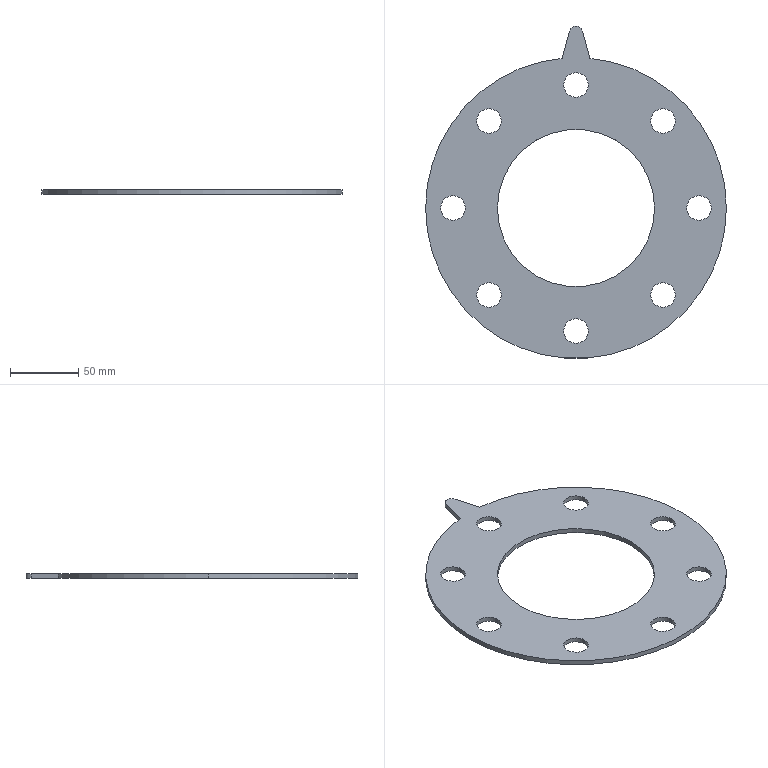Part | SolidWorks | features Extrusion 1 | 1 solid | 26 faces | box 220 x 243.233 x 3.5 mm | volume 90689 mm3 | cylinder 22 | plane 4 | commonest cylinder face diameters 18 x16 220 x3 115 x2 10 x1
STEP:
#1=CARTESIAN_POINT('',(-72.64,63.64,3.5));
#2=VERTEX_POINT('',#1);
#3=CARTESIAN_POINT('',(-54.64,63.64,3.5));
#4=VERTEX_POINT('',#3);
#5=CARTESIAN_POINT('',(-63.64,63.64,3.5));
#6=DIRECTION('',(0.,0.,1.));
#7=DIRECTION('',(1.,0.,0.));
#8=AXIS2_PLACEMENT_3D('',#5,#6,#7);
#9=CIRCLE('',#8,9.);
#10=EDGE_CURVE('',#2,#4,#9,.T.);
#11=ORIENTED_EDGE('',*,*,#10,.T.);
#12=CARTESIAN_POINT('',(-54.64,63.64,0.));
#13=VERTEX_POINT('',#12);
#14=CARTESIAN_POINT('',(-54.64,63.64,3.5));
#15=DIRECTION('',(0.,0.,-1.));
#16=VECTOR('',#15,1000.);
#17=LINE('',#14,#16);
#18=EDGE_CURVE('',#4,#13,#17,.T.);
#19=ORIENTED_EDGE('',*,*,#18,.T.);
#20=CARTESIAN_POINT('',(-72.64,63.64,0.));
#21=VERTEX_POINT('',#20);
#22=CARTESIAN_POINT('',(-63.64,63.64,0.));
#23=DIRECTION('',(0.,0.,1.));
#24=DIRECTION('',(1.,0.,0.));
#25=AXIS2_PLACEMENT_3D('',#22,#23,#24);
#26=CIRCLE('',#25,9.);
#27=EDGE_CURVE('',#21,#13,#26,.T.);
#28=ORIENTED_EDGE('',*,*,#27,.F.);
#29=CARTESIAN_POINT('',(-72.64,63.64,3.5));
#30=DIRECTION('',(0.,0.,-1.));
#31=VECTOR('',#30,1000.);
#32=LINE('',#29,#31);
#33=EDGE_CURVE('',#2,#21,#32,.T.);
#34=ORIENTED_EDGE('',*,*,#33,.F.);
#35=EDGE_LOOP('',(#11,#19,#28,#34));
#36=FACE_OUTER_BOUND('',#35,.T.);
#37=CARTESIAN_POINT('',(-63.64,63.64,3.5));
#38=DIRECTION('',(0.,0.,-1.));
#39=DIRECTION('',(-1.,0.,0.));
#40=AXIS2_PLACEMENT_3D('',#37,#38,#39);
#41=CYLINDRICAL_SURFACE('',#40,9.);
#42=ADVANCED_FACE('',(#36),#41,.F.);
#43=CARTESIAN_POINT('',(-99.,0.,3.5));
#44=VERTEX_POINT('',#43);
#45=CARTESIAN_POINT('',(-81.,0.,3.5));
#46=VERTEX_POINT('',#45);
#47=CARTESIAN_POINT('',(-90.,0.,3.5));
#48=DIRECTION('',(0.,0.,1.));
#49=DIRECTION('',(1.,0.,0.));
#50=AXIS2_PLACEMENT_3D('',#47,#48,#49);
#51=CIRCLE('',#50,9.);
#52=EDGE_CURVE('',#44,#46,#51,.T.);
#53=ORIENTED_EDGE('',*,*,#52,.T.);
#54=CARTESIAN_POINT('',(-81.,0.,0.));
#55=VERTEX_POINT('',#54);
#56=CARTESIAN_POINT('',(-81.,0.,3.5));
#57=DIRECTION('',(0.,0.,-1.));
#58=VECTOR('',#57,1000.);
#59=LINE('',#56,#58);
#60=EDGE_CURVE('',#46,#55,#59,.T.);
#61=ORIENTED_EDGE('',*,*,#60,.T.);
#62=CARTESIAN_POINT('',(-99.,0.,0.));
#63=VERTEX_POINT('',#62);
#64=CARTESIAN_POINT('',(-90.,0.,0.));
#65=DIRECTION('',(0.,0.,1.));
#66=DIRECTION('',(1.,0.,0.));
#67=AXIS2_PLACEMENT_3D('',#64,#65,#66);
#68=CIRCLE('',#67,9.);
#69=EDGE_CURVE('',#63,#55,#68,.T.);
#70=ORIENTED_EDGE('',*,*,#69,.F.);
#71=CARTESIAN_POINT('',(-99.,0.,3.5));
#72=DIRECTION('',(0.,0.,-1.));
#73=VECTOR('',#72,1000.);
#74=LINE('',#71,#73);
#75=EDGE_CURVE('',#44,#63,#74,.T.);
#76=ORIENTED_EDGE('',*,*,#75,.F.);
#77=EDGE_LOOP('',(#53,#61,#70,#76));
#78=FACE_OUTER_BOUND('',#77,.T.);
#79=CARTESIAN_POINT('',(-90.,0.,3.5));
#80=DIRECTION('',(0.,0.,-1.));
#81=DIRECTION('',(-1.,0.,0.));
#82=AXIS2_PLACEMENT_3D('',#79,#80,#81);
#83=CYLINDRICAL_SURFACE('',#82,9.);
#84=ADVANCED_FACE('',(#78),#83,.F.);
#85=CARTESIAN_POINT('',(-72.64,-63.64,3.5));
#86=VERTEX_POINT('',#85);
#87=CARTESIAN_POINT('',(-54.64,-63.64,3.5));
#88=VERTEX_POINT('',#87);
#89=CARTESIAN_POINT('',(-63.64,-63.64,3.5));
#90=DIRECTION('',(0.,0.,1.));
#91=DIRECTION('',(1.,0.,0.));
#92=AXIS2_PLACEMENT_3D('',#89,#90,#91);
#93=CIRCLE('',#92,9.);
#94=EDGE_CURVE('',#86,#88,#93,.T.);
#95=ORIENTED_EDGE('',*,*,#94,.T.);
#96=CARTESIAN_POINT('',(-54.64,-63.64,0.));
#97=VERTEX_POINT('',#96);
#98=CARTESIAN_POINT('',(-54.64,-63.64,3.5));
#99=DIRECTION('',(0.,0.,-1.));
#100=VECTOR('',#99,1000.);
#101=LINE('',#98,#100);
#102=EDGE_CURVE('',#88,#97,#101,.T.);
#103=ORIENTED_EDGE('',*,*,#102,.T.);
#104=CARTESIAN_POINT('',(-72.64,-63.64,0.));
#105=VERTEX_POINT('',#104);
#106=CARTESIAN_POINT('',(-63.64,-63.64,0.));
#107=DIRECTION('',(0.,0.,1.));
#108=DIRECTION('',(1.,0.,0.));
#109=AXIS2_PLACEMENT_3D('',#106,#107,#108);
#110=CIRCLE('',#109,9.);
#111=EDGE_CURVE('',#105,#97,#110,.T.);
#112=ORIENTED_EDGE('',*,*,#111,.F.);
#113=CARTESIAN_POINT('',(-72.64,-63.64,3.5));
#114=DIRECTION('',(0.,0.,-1.));
#115=VECTOR('',#114,1000.);
#116=LINE('',#113,#115);
#117=EDGE_CURVE('',#86,#105,#116,.T.);
#118=ORIENTED_EDGE('',*,*,#117,.F.);
#119=EDGE_LOOP('',(#95,#103,#112,#118));
#120=FACE_OUTER_BOUND('',#119,.T.);
#121=CARTESIAN_POINT('',(-63.64,-63.64,3.5));
#122=DIRECTION('',(0.,0.,-1.));
#123=DIRECTION('',(-1.,0.,0.));
#124=AXIS2_PLACEMENT_3D('',#121,#122,#123);
#125=CYLINDRICAL_SURFACE('',#124,9.);
#126=ADVANCED_FACE('',(#120),#125,.F.);
#127=CARTESIAN_POINT('',(-9.,-90.,3.5));
#128=VERTEX_POINT('',#127);
#129=CARTESIAN_POINT('',(9.,-90.,3.5));
#130=VERTEX_POINT('',#129);
#131=CARTESIAN_POINT('',(0.,-90.,3.5));
#132=DIRECTION('',(0.,0.,1.));
#133=DIRECTION('',(1.,0.,0.));
#134=AXIS2_PLACEMENT_3D('',#131,#132,#133);
#135=CIRCLE('',#134,9.);
#136=EDGE_CURVE('',#128,#130,#135,.T.);
#137=ORIENTED_EDGE('',*,*,#136,.T.);
#138=CARTESIAN_POINT('',(9.,-90.,0.));
#139=VERTEX_POINT('',#138);
#140=CARTESIAN_POINT('',(9.,-90.,3.5));
#141=DIRECTION('',(0.,0.,-1.));
#142=VECTOR('',#141,1000.);
#143=LINE('',#140,#142);
#144=EDGE_CURVE('',#130,#139,#143,.T.);
#145=ORIENTED_EDGE('',*,*,#144,.T.);
#146=CARTESIAN_POINT('',(-9.,-90.,0.));
#147=VERTEX_POINT('',#146);
#148=CARTESIAN_POINT('',(0.,-90.,0.));
#149=DIRECTION('',(0.,0.,1.));
#150=DIRECTION('',(1.,0.,0.));
#151=AXIS2_PLACEMENT_3D('',#148,#149,#150);
#152=CIRCLE('',#151,9.);
#153=EDGE_CURVE('',#147,#139,#152,.T.);
#154=ORIENTED_EDGE('',*,*,#153,.F.);
#155=CARTESIAN_POINT('',(-9.,-90.,3.5));
#156=DIRECTION('',(0.,0.,-1.));
#157=VECTOR('',#156,1000.);
#158=LINE('',#155,#157);
#159=EDGE_CURVE('',#128,#147,#158,.T.);
#160=ORIENTED_EDGE('',*,*,#159,.F.);
#161=EDGE_LOOP('',(#137,#145,#154,#160));
#162=FACE_OUTER_BOUND('',#161,.T.);
#163=CARTESIAN_POINT('',(0.,-90.,3.5));
#164=DIRECTION('',(0.,0.,-1.));
#165=DIRECTION('',(-1.,0.,0.));
#166=AXIS2_PLACEMENT_3D('',#163,#164,#165);
#167=CYLINDRICAL_SURFACE('',#166,9.);
#168=ADVANCED_FACE('',(#162),#167,.F.);
#169=CARTESIAN_POINT('',(54.64,-63.64,3.5));
#170=VERTEX_POINT('',#169);
#171=CARTESIAN_POINT('',(72.64,-63.64,3.5));
#172=VERTEX_POINT('',#171);
#173=CARTESIAN_POINT('',(63.64,-63.64,3.5));
#174=DIRECTION('',(0.,0.,1.));
#175=DIRECTION('',(1.,0.,0.));
#176=AXIS2_PLACEMENT_3D('',#173,#174,#175);
#177=CIRCLE('',#176,9.);
#178=EDGE_CURVE('',#170,#172,#177,.T.);
#179=ORIENTED_EDGE('',*,*,#178,.T.);
#180=CARTESIAN_POINT('',(72.64,-63.64,0.));
#181=VERTEX_POINT('',#180);
#182=CARTESIAN_POINT('',(72.64,-63.64,3.5));
#183=DIRECTION('',(0.,0.,-1.));
#184=VECTOR('',#183,1000.);
#185=LINE('',#182,#184);
#186=EDGE_CURVE('',#172,#181,#185,.T.);
#187=ORIENTED_EDGE('',*,*,#186,.T.);
#188=CARTESIAN_POINT('',(54.64,-63.64,0.));
#189=VERTEX_POINT('',#188);
#190=CARTESIAN_POINT('',(63.64,-63.64,0.));
#191=DIRECTION('',(0.,0.,1.));
#192=DIRECTION('',(1.,0.,0.));
#193=AXIS2_PLACEMENT_3D('',#190,#191,#192);
#194=CIRCLE('',#193,9.);
#195=EDGE_CURVE('',#189,#181,#194,.T.);
#196=ORIENTED_EDGE('',*,*,#195,.F.);
#197=CARTESIAN_POINT('',(54.64,-63.64,3.5));
#198=DIRECTION('',(0.,0.,-1.));
#199=VECTOR('',#198,1000.);
#200=LINE('',#197,#199);
#201=EDGE_CURVE('',#170,#189,#200,.T.);
#202=ORIENTED_EDGE('',*,*,#201,.F.);
#203=EDGE_LOOP('',(#179,#187,#196,#202));
#204=FACE_OUTER_BOUND('',#203,.T.);
#205=CARTESIAN_POINT('',(63.64,-63.64,3.5));
#206=DIRECTION('',(0.,0.,-1.));
#207=DIRECTION('',(-1.,0.,0.));
#208=AXIS2_PLACEMENT_3D('',#205,#206,#207);
#209=CYLINDRICAL_SURFACE('',#208,9.);
#210=ADVANCED_FACE('',(#204),#209,.F.);
#211=CARTESIAN_POINT('',(81.,0.,3.5));
#212=VERTEX_POINT('',#211);
#213=CARTESIAN_POINT('',(99.,0.,3.5));
#214=VERTEX_POINT('',#213);
#215=CARTESIAN_POINT('',(90.,0.,3.5));
#216=DIRECTION('',(0.,0.,1.));
#217=DIRECTION('',(1.,0.,0.));
#218=AXIS2_PLACEMENT_3D('',#215,#216,#217);
#219=CIRCLE('',#218,9.);
#220=EDGE_CURVE('',#212,#214,#219,.T.);
#221=ORIENTED_EDGE('',*,*,#220,.T.);
#222=CARTESIAN_POINT('',(99.,0.,0.));
#223=VERTEX_POINT('',#222);
#224=CARTESIAN_POINT('',(99.,0.,3.5));
#225=DIRECTION('',(0.,0.,-1.));
#226=VECTOR('',#225,1000.);
#227=LINE('',#224,#226);
#228=EDGE_CURVE('',#214,#223,#227,.T.);
#229=ORIENTED_EDGE('',*,*,#228,.T.);
#230=CARTESIAN_POINT('',(81.,0.,0.));
#231=VERTEX_POINT('',#230);
#232=CARTESIAN_POINT('',(90.,0.,0.));
#233=DIRECTION('',(0.,0.,1.));
#234=DIRECTION('',(1.,0.,0.));
#235=AXIS2_PLACEMENT_3D('',#232,#233,#234);
#236=CIRCLE('',#235,9.);
#237=EDGE_CURVE('',#231,#223,#236,.T.);
#238=ORIENTED_EDGE('',*,*,#237,.F.);
#239=CARTESIAN_POINT('',(81.,0.,3.5));
#240=DIRECTION('',(0.,0.,-1.));
#241=VECTOR('',#240,1000.);
#242=LINE('',#239,#241);
#243=EDGE_CURVE('',#212,#231,#242,.T.);
#244=ORIENTED_EDGE('',*,*,#243,.F.);
#245=EDGE_LOOP('',(#221,#229,#238,#244));
#246=FACE_OUTER_BOUND('',#245,.T.);
#247=CARTESIAN_POINT('',(90.,0.,3.5));
#248=DIRECTION('',(0.,0.,-1.));
#249=DIRECTION('',(-1.,0.,0.));
#250=AXIS2_PLACEMENT_3D('',#247,#248,#249);
#251=CYLINDRICAL_SURFACE('',#250,9.);
#252=ADVANCED_FACE('',(#246),#251,.F.);
#253=CARTESIAN_POINT('',(54.64,63.64,3.5));
#254=VERTEX_POINT('',#253);
#255=CARTESIAN_POINT('',(72.64,63.64,3.5));
#256=VERTEX_POINT('',#255);
#257=CARTESIAN_POINT('',(63.64,63.64,3.5));
#258=DIRECTION('',(0.,0.,1.));
#259=DIRECTION('',(1.,0.,0.));
#260=AXIS2_PLACEMENT_3D('',#257,#258,#259);
#261=CIRCLE('',#260,9.);
#262=EDGE_CURVE('',#254,#256,#261,.T.);
#263=ORIENTED_EDGE('',*,*,#262,.T.);
#264=CARTESIAN_POINT('',(72.64,63.64,0.));
#265=VERTEX_POINT('',#264);
#266=CARTESIAN_POINT('',(72.64,63.64,3.5));
#267=DIRECTION('',(0.,0.,-1.));
#268=VECTOR('',#267,1000.);
#269=LINE('',#266,#268);
#270=EDGE_CURVE('',#256,#265,#269,.T.);
#271=ORIENTED_EDGE('',*,*,#270,.T.);
#272=CARTESIAN_POINT('',(54.64,63.64,0.));
#273=VERTEX_POINT('',#272);
#274=CARTESIAN_POINT('',(63.64,63.64,0.));
#275=DIRECTION('',(0.,0.,1.));
#276=DIRECTION('',(1.,0.,0.));
#277=AXIS2_PLACEMENT_3D('',#274,#275,#276);
#278=CIRCLE('',#277,9.);
#279=EDGE_CURVE('',#273,#265,#278,.T.);
#280=ORIENTED_EDGE('',*,*,#279,.F.);
#281=CARTESIAN_POINT('',(54.64,63.64,3.5));
#282=DIRECTION('',(0.,0.,-1.));
#283=VECTOR('',#282,1000.);
#284=LINE('',#281,#283);
#285=EDGE_CURVE('',#254,#273,#284,.T.);
#286=ORIENTED_EDGE('',*,*,#285,.F.);
#287=EDGE_LOOP('',(#263,#271,#280,#286));
#288=FACE_OUTER_BOUND('',#287,.T.);
#289=CARTESIAN_POINT('',(63.64,63.64,3.5));
#290=DIRECTION('',(0.,0.,-1.));
#291=DIRECTION('',(-1.,0.,0.));
#292=AXIS2_PLACEMENT_3D('',#289,#290,#291);
#293=CYLINDRICAL_SURFACE('',#292,9.);
#294=ADVANCED_FACE('',(#288),#293,.F.);
#295=CARTESIAN_POINT('',(-9.,90.,3.5));
#296=VERTEX_POINT('',#295);
#297=CARTESIAN_POINT('',(9.,90.,3.5));
#298=VERTEX_POINT('',#297);
#299=CARTESIAN_POINT('',(0.,90.,3.5));
#300=DIRECTION('',(0.,0.,1.));
#301=DIRECTION('',(1.,0.,0.));
#302=AXIS2_PLACEMENT_3D('',#299,#300,#301);
#303=CIRCLE('',#302,9.);
#304=EDGE_CURVE('',#296,#298,#303,.T.);
#305=ORIENTED_EDGE('',*,*,#304,.T.);
#306=CARTESIAN_POINT('',(9.,90.,0.));
#307=VERTEX_POINT('',#306);
#308=CARTESIAN_POINT('',(9.,90.,3.5));
#309=DIRECTION('',(0.,0.,-1.));
#310=VECTOR('',#309,1000.);
#311=LINE('',#308,#310);
#312=EDGE_CURVE('',#298,#307,#311,.T.);
#313=ORIENTED_EDGE('',*,*,#312,.T.);
#314=CARTESIAN_POINT('',(-9.,90.,0.));
#315=VERTEX_POINT('',#314);
#316=CARTESIAN_POINT('',(0.,90.,0.));
#317=DIRECTION('',(0.,0.,1.));
#318=DIRECTION('',(1.,0.,0.));
#319=AXIS2_PLACEMENT_3D('',#316,#317,#318);
#320=CIRCLE('',#319,9.);
#321=EDGE_CURVE('',#315,#307,#320,.T.);
#322=ORIENTED_EDGE('',*,*,#321,.F.);
#323=CARTESIAN_POINT('',(-9.,90.,3.5));
#324=DIRECTION('',(0.,0.,-1.));
#325=VECTOR('',#324,1000.);
#326=LINE('',#323,#325);
#327=EDGE_CURVE('',#296,#315,#326,.T.);
#328=ORIENTED_EDGE('',*,*,#327,.F.);
#329=EDGE_LOOP('',(#305,#313,#322,#328));
#330=FACE_OUTER_BOUND('',#329,.T.);
#331=CARTESIAN_POINT('',(0.,90.,3.5));
#332=DIRECTION('',(0.,0.,-1.));
#333=DIRECTION('',(-1.,0.,0.));
#334=AXIS2_PLACEMENT_3D('',#331,#332,#333);
#335=CYLINDRICAL_SURFACE('',#334,9.);
#336=ADVANCED_FACE('',(#330),#335,.F.);
#337=CARTESIAN_POINT('',(-57.5,0.,3.5));
#338=VERTEX_POINT('',#337);
#339=CARTESIAN_POINT('',(57.5,0.,3.5));
#340=VERTEX_POINT('',#339);
#341=CARTESIAN_POINT('',(0.,0.,3.5));
#342=DIRECTION('',(0.,0.,1.));
#343=DIRECTION('',(1.,0.,0.));
#344=AXIS2_PLACEMENT_3D('',#341,#342,#343);
#345=CIRCLE('',#344,57.5);
#346=EDGE_CURVE('',#338,#340,#345,.T.);
#347=ORIENTED_EDGE('',*,*,#346,.T.);
#348=CARTESIAN_POINT('',(57.5,0.,0.));
#349=VERTEX_POINT('',#348);
#350=CARTESIAN_POINT('',(57.5,0.,3.5));
#351=DIRECTION('',(0.,0.,-1.));
#352=VECTOR('',#351,1000.);
#353=LINE('',#350,#352);
#354=EDGE_CURVE('',#340,#349,#353,.T.);
#355=ORIENTED_EDGE('',*,*,#354,.T.);
#356=CARTESIAN_POINT('',(-57.5,0.,0.));
#357=VERTEX_POINT('',#356);
#358=CARTESIAN_POINT('',(0.,0.,0.));
#359=DIRECTION('',(0.,0.,1.));
#360=DIRECTION('',(1.,0.,0.));
#361=AXIS2_PLACEMENT_3D('',#358,#359,#360);
#362=CIRCLE('',#361,57.5);
#363=EDGE_CURVE('',#357,#349,#362,.T.);
#364=ORIENTED_EDGE('',*,*,#363,.F.);
#365=CARTESIAN_POINT('',(-57.5,0.,3.5));
#366=DIRECTION('',(0.,0.,-1.));
#367=VECTOR('',#366,1000.);
#368=LINE('',#365,#367);
#369=EDGE_CURVE('',#338,#357,#368,.T.);
#370=ORIENTED_EDGE('',*,*,#369,.F.);
#371=EDGE_LOOP('',(#347,#355,#364,#370));
#372=FACE_OUTER_BOUND('',#371,.T.);
#373=CARTESIAN_POINT('',(0.,0.,3.5));
#374=DIRECTION('',(0.,0.,-1.));
#375=DIRECTION('',(-1.,0.,0.));
#376=AXIS2_PLACEMENT_3D('',#373,#374,#375);
#377=CYLINDRICAL_SURFACE('',#376,57.5);
#378=ADVANCED_FACE('',(#372),#377,.F.);
#379=CARTESIAN_POINT('',(110.,0.,3.5));
#380=VERTEX_POINT('',#379);
#381=CARTESIAN_POINT('',(10.189,109.527,3.5));
#382=VERTEX_POINT('',#381);
#383=CARTESIAN_POINT('',(0.,0.,3.5));
#384=DIRECTION('',(0.,0.,1.));
#385=DIRECTION('',(1.,0.,0.));
#386=AXIS2_PLACEMENT_3D('',#383,#384,#385);
#387=CIRCLE('',#386,110.);
#388=EDGE_CURVE('',#380,#382,#387,.T.);
#389=ORIENTED_EDGE('',*,*,#388,.F.);
#390=CARTESIAN_POINT('',(110.,0.,0.));
#391=VERTEX_POINT('',#390);
#392=CARTESIAN_POINT('',(110.,0.,3.5));
#393=DIRECTION('',(0.,0.,-1.));
#394=VECTOR('',#393,1000.);
#395=LINE('',#392,#394);
#396=EDGE_CURVE('',#380,#391,#395,.T.);
#397=ORIENTED_EDGE('',*,*,#396,.T.);
#398=CARTESIAN_POINT('',(10.189,109.527,0.));
#399=VERTEX_POINT('',#398);
#400=CARTESIAN_POINT('',(0.,0.,0.));
#401=DIRECTION('',(0.,0.,1.));
#402=DIRECTION('',(1.,0.,0.));
#403=AXIS2_PLACEMENT_3D('',#400,#401,#402);
#404=CIRCLE('',#403,110.);
#405=EDGE_CURVE('',#391,#399,#404,.T.);
#406=ORIENTED_EDGE('',*,*,#405,.T.);
#407=CARTESIAN_POINT('',(10.189,109.527,3.5));
#408=DIRECTION('',(0.,0.,-1.));
#409=VECTOR('',#408,1000.);
#410=LINE('',#407,#409);
#411=EDGE_CURVE('',#382,#399,#410,.T.);
#412=ORIENTED_EDGE('',*,*,#411,.F.);
#413=EDGE_LOOP('',(#389,#397,#406,#412));
#414=FACE_OUTER_BOUND('',#413,.T.);
#415=CARTESIAN_POINT('',(0.,0.,3.5));
#416=DIRECTION('',(0.,0.,-1.));
#417=DIRECTION('',(-1.,0.,0.));
#418=AXIS2_PLACEMENT_3D('',#415,#416,#417);
#419=CYLINDRICAL_SURFACE('',#418,110.);
#420=ADVANCED_FACE('',(#414),#419,.T.);
#421=ORIENTED_EDGE('',*,*,#396,.F.);
#422=CARTESIAN_POINT('',(-110.,0.,3.5));
#423=VERTEX_POINT('',#422);
#424=CARTESIAN_POINT('',(0.,0.,3.5));
#425=DIRECTION('',(0.,0.,1.));
#426=DIRECTION('',(1.,0.,0.));
#427=AXIS2_PLACEMENT_3D('',#424,#425,#426);
#428=CIRCLE('',#427,110.);
#429=EDGE_CURVE('',#423,#380,#428,.T.);
#430=ORIENTED_EDGE('',*,*,#429,.F.);
#431=CARTESIAN_POINT('',(-110.,0.,0.));
#432=VERTEX_POINT('',#431);
#433=CARTESIAN_POINT('',(-110.,0.,3.5));
#434=DIRECTION('',(0.,0.,-1.));
#435=VECTOR('',#434,1000.);
#436=LINE('',#433,#435);
#437=EDGE_CURVE('',#423,#432,#436,.T.);
#438=ORIENTED_EDGE('',*,*,#437,.T.);
#439=CARTESIAN_POINT('',(0.,0.,0.));
#440=DIRECTION('',(0.,0.,1.));
#441=DIRECTION('',(1.,0.,0.));
#442=AXIS2_PLACEMENT_3D('',#439,#440,#441);
#443=CIRCLE('',#442,110.);
#444=EDGE_CURVE('',#432,#391,#443,.T.);
#445=ORIENTED_EDGE('',*,*,#444,.T.);
#446=EDGE_LOOP('',(#421,#430,#438,#445));
#447=FACE_OUTER_BOUND('',#446,.T.);
#448=CARTESIAN_POINT('',(0.,0.,3.5));
#449=DIRECTION('',(0.,0.,-1.));
#450=DIRECTION('',(-1.,0.,0.));
#451=AXIS2_PLACEMENT_3D('',#448,#449,#450);
#452=CYLINDRICAL_SURFACE('',#451,110.);
#453=ADVANCED_FACE('',(#447),#452,.T.);
#454=ORIENTED_EDGE('',*,*,#52,.F.);
#455=CARTESIAN_POINT('',(-90.,0.,3.5));
#456=DIRECTION('',(0.,0.,1.));
#457=DIRECTION('',(1.,0.,0.));
#458=AXIS2_PLACEMENT_3D('',#455,#456,#457);
#459=CIRCLE('',#458,9.);
#460=EDGE_CURVE('',#46,#44,#459,.T.);
#461=ORIENTED_EDGE('',*,*,#460,.F.);
#462=EDGE_LOOP('',(#454,#461));
#463=FACE_BOUND('',#462,.T.);
#464=ORIENTED_EDGE('',*,*,#136,.F.);
#465=CARTESIAN_POINT('',(0.,-90.,3.5));
#466=DIRECTION('',(0.,0.,1.));
#467=DIRECTION('',(1.,0.,0.));
#468=AXIS2_PLACEMENT_3D('',#465,#466,#467);
#469=CIRCLE('',#468,9.);
#470=EDGE_CURVE('',#130,#128,#469,.T.);
#471=ORIENTED_EDGE('',*,*,#470,.F.);
#472=EDGE_LOOP('',(#464,#471));
#473=FACE_BOUND('',#472,.T.);
#474=ORIENTED_EDGE('',*,*,#220,.F.);
#475=CARTESIAN_POINT('',(90.,0.,3.5));
#476=DIRECTION('',(0.,0.,1.));
#477=DIRECTION('',(1.,0.,0.));
#478=AXIS2_PLACEMENT_3D('',#475,#476,#477);
#479=CIRCLE('',#478,9.);
#480=EDGE_CURVE('',#214,#212,#479,.T.);
#481=ORIENTED_EDGE('',*,*,#480,.F.);
#482=EDGE_LOOP('',(#474,#481));
#483=FACE_BOUND('',#482,.T.);
#484=ORIENTED_EDGE('',*,*,#304,.F.);
#485=CARTESIAN_POINT('',(0.,90.,3.5));
#486=DIRECTION('',(0.,0.,1.));
#487=DIRECTION('',(1.,0.,0.));
#488=AXIS2_PLACEMENT_3D('',#485,#486,#487);
#489=CIRCLE('',#488,9.);
#490=EDGE_CURVE('',#298,#296,#489,.T.);
#491=ORIENTED_EDGE('',*,*,#490,.F.);
#492=EDGE_LOOP('',(#484,#491));
#493=FACE_BOUND('',#492,.T.);
#494=CARTESIAN_POINT('',(-10.189,109.527,3.5));
#495=VERTEX_POINT('',#494);
#496=CARTESIAN_POINT('',(0.,0.,3.5));
#497=DIRECTION('',(0.,0.,1.));
#498=DIRECTION('',(1.,0.,0.));
#499=AXIS2_PLACEMENT_3D('',#496,#497,#498);
#500=CIRCLE('',#499,110.);
#501=EDGE_CURVE('',#495,#423,#500,.T.);
#502=ORIENTED_EDGE('',*,*,#501,.T.);
#503=ORIENTED_EDGE('',*,*,#429,.T.);
#504=ORIENTED_EDGE('',*,*,#388,.T.);
#505=CARTESIAN_POINT('',(4.83,129.527,3.5));
#506=VERTEX_POINT('',#505);
#507=CARTESIAN_POINT('',(4.83,129.527,3.5));
#508=DIRECTION('',(-0.2588,0.9659,0.));
#509=VECTOR('',#508,1000.);
#510=LINE('',#507,#509);
#511=EDGE_CURVE('',#382,#506,#510,.T.);
#512=ORIENTED_EDGE('',*,*,#511,.T.);
#513=CARTESIAN_POINT('',(-4.83,129.527,3.5));
#514=VERTEX_POINT('',#513);
#515=CARTESIAN_POINT('',(0.,128.233,3.5));
#516=DIRECTION('',(0.,0.,1.));
#517=DIRECTION('',(-1.,0.,0.));
#518=AXIS2_PLACEMENT_3D('',#515,#516,#517);
#519=CIRCLE('',#518,5.);
#520=EDGE_CURVE('',#506,#514,#519,.T.);
#521=ORIENTED_EDGE('',*,*,#520,.T.);
#522=CARTESIAN_POINT('',(-4.83,129.527,3.5));
#523=DIRECTION('',(-0.2588,-0.9659,0.));
#524=VECTOR('',#523,1000.);
#525=LINE('',#522,#524);
#526=EDGE_CURVE('',#514,#495,#525,.T.);
#527=ORIENTED_EDGE('',*,*,#526,.T.);
#528=EDGE_LOOP('',(#502,#503,#504,#512,#521,#527));
#529=FACE_OUTER_BOUND('',#528,.T.);
#530=ORIENTED_EDGE('',*,*,#346,.F.);
#531=CARTESIAN_POINT('',(0.,0.,3.5));
#532=DIRECTION('',(0.,0.,1.));
#533=DIRECTION('',(1.,0.,0.));
#534=AXIS2_PLACEMENT_3D('',#531,#532,#533);
#535=CIRCLE('',#534,57.5);
#536=EDGE_CURVE('',#340,#338,#535,.T.);
#537=ORIENTED_EDGE('',*,*,#536,.F.);
#538=EDGE_LOOP('',(#530,#537));
#539=FACE_BOUND('',#538,.T.);
#540=ORIENTED_EDGE('',*,*,#262,.F.);
#541=CARTESIAN_POINT('',(63.64,63.64,3.5));
#542=DIRECTION('',(0.,0.,1.));
#543=DIRECTION('',(1.,0.,0.));
#544=AXIS2_PLACEMENT_3D('',#541,#542,#543);
#545=CIRCLE('',#544,9.);
#546=EDGE_CURVE('',#256,#254,#545,.T.);
#547=ORIENTED_EDGE('',*,*,#546,.F.);
#548=EDGE_LOOP('',(#540,#547));
#549=FACE_BOUND('',#548,.T.);
#550=ORIENTED_EDGE('',*,*,#178,.F.);
#551=CARTESIAN_POINT('',(63.64,-63.64,3.5));
#552=DIRECTION('',(0.,0.,1.));
#553=DIRECTION('',(1.,0.,0.));
#554=AXIS2_PLACEMENT_3D('',#551,#552,#553);
#555=CIRCLE('',#554,9.);
#556=EDGE_CURVE('',#172,#170,#555,.T.);
#557=ORIENTED_EDGE('',*,*,#556,.F.);
#558=EDGE_LOOP('',(#550,#557));
#559=FACE_BOUND('',#558,.T.);
#560=ORIENTED_EDGE('',*,*,#94,.F.);
#561=CARTESIAN_POINT('',(-63.64,-63.64,3.5));
#562=DIRECTION('',(0.,0.,1.));
#563=DIRECTION('',(1.,0.,0.));
#564=AXIS2_PLACEMENT_3D('',#561,#562,#563);
#565=CIRCLE('',#564,9.);
#566=EDGE_CURVE('',#88,#86,#565,.T.);
#567=ORIENTED_EDGE('',*,*,#566,.F.);
#568=EDGE_LOOP('',(#560,#567));
#569=FACE_BOUND('',#568,.T.);
#570=ORIENTED_EDGE('',*,*,#10,.F.);
#571=CARTESIAN_POINT('',(-63.64,63.64,3.5));
#572=DIRECTION('',(0.,0.,1.));
#573=DIRECTION('',(1.,0.,0.));
#574=AXIS2_PLACEMENT_3D('',#571,#572,#573);
#575=CIRCLE('',#574,9.);
#576=EDGE_CURVE('',#4,#2,#575,.T.);
#577=ORIENTED_EDGE('',*,*,#576,.F.);
#578=EDGE_LOOP('',(#570,#577));
#579=FACE_BOUND('',#578,.T.);
#580=CARTESIAN_POINT('',(0.,0.,3.5));
#581=DIRECTION('',(0.,0.,1.));
#582=DIRECTION('',(1.,0.,0.));
#583=AXIS2_PLACEMENT_3D('',#580,#581,#582);
#584=PLANE('',#583);
#585=ADVANCED_FACE('',(#463,#473,#483,#493,#529,#539,#549,#559,#569,#579),#584,.T.);
#586=CARTESIAN_POINT('',(-10.189,109.527,0.));
#587=VERTEX_POINT('',#586);
#588=CARTESIAN_POINT('',(0.,0.,0.));
#589=DIRECTION('',(0.,0.,1.));
#590=DIRECTION('',(1.,0.,0.));
#591=AXIS2_PLACEMENT_3D('',#588,#589,#590);
#592=CIRCLE('',#591,110.);
#593=EDGE_CURVE('',#587,#432,#592,.T.);
#594=ORIENTED_EDGE('',*,*,#593,.F.);
#595=CARTESIAN_POINT('',(-4.83,129.527,0.));
#596=VERTEX_POINT('',#595);
#597=CARTESIAN_POINT('',(-4.83,129.527,0.));
#598=DIRECTION('',(-0.2588,-0.9659,0.));
#599=VECTOR('',#598,1000.);
#600=LINE('',#597,#599);
#601=EDGE_CURVE('',#596,#587,#600,.T.);
#602=ORIENTED_EDGE('',*,*,#601,.F.);
#603=CARTESIAN_POINT('',(4.83,129.527,0.));
#604=VERTEX_POINT('',#603);
#605=CARTESIAN_POINT('',(0.,128.233,0.));
#606=DIRECTION('',(0.,0.,1.));
#607=DIRECTION('',(-1.,0.,0.));
#608=AXIS2_PLACEMENT_3D('',#605,#606,#607);
#609=CIRCLE('',#608,5.);
#610=EDGE_CURVE('',#604,#596,#609,.T.);
#611=ORIENTED_EDGE('',*,*,#610,.F.);
#612=CARTESIAN_POINT('',(4.83,129.527,0.));
#613=DIRECTION('',(-0.2588,0.9659,0.));
#614=VECTOR('',#613,1000.);
#615=LINE('',#612,#614);
#616=EDGE_CURVE('',#399,#604,#615,.T.);
#617=ORIENTED_EDGE('',*,*,#616,.F.);
#618=ORIENTED_EDGE('',*,*,#405,.F.);
#619=ORIENTED_EDGE('',*,*,#444,.F.);
#620=EDGE_LOOP('',(#594,#602,#611,#617,#618,#619));
#621=FACE_OUTER_BOUND('',#620,.T.);
#622=ORIENTED_EDGE('',*,*,#363,.T.);
#623=CARTESIAN_POINT('',(0.,0.,0.));
#624=DIRECTION('',(0.,0.,1.));
#625=DIRECTION('',(1.,0.,0.));
#626=AXIS2_PLACEMENT_3D('',#623,#624,#625);
#627=CIRCLE('',#626,57.5);
#628=EDGE_CURVE('',#349,#357,#627,.T.);
#629=ORIENTED_EDGE('',*,*,#628,.T.);
#630=EDGE_LOOP('',(#622,#629));
#631=FACE_BOUND('',#630,.T.);
#632=ORIENTED_EDGE('',*,*,#321,.T.);
#633=CARTESIAN_POINT('',(0.,90.,0.));
#634=DIRECTION('',(0.,0.,1.));
#635=DIRECTION('',(1.,0.,0.));
#636=AXIS2_PLACEMENT_3D('',#633,#634,#635);
#637=CIRCLE('',#636,9.);
#638=EDGE_CURVE('',#307,#315,#637,.T.);
#639=ORIENTED_EDGE('',*,*,#638,.T.);
#640=EDGE_LOOP('',(#632,#639));
#641=FACE_BOUND('',#640,.T.);
#642=ORIENTED_EDGE('',*,*,#279,.T.);
#643=CARTESIAN_POINT('',(63.64,63.64,0.));
#644=DIRECTION('',(0.,0.,1.));
#645=DIRECTION('',(1.,0.,0.));
#646=AXIS2_PLACEMENT_3D('',#643,#644,#645);
#647=CIRCLE('',#646,9.);
#648=EDGE_CURVE('',#265,#273,#647,.T.);
#649=ORIENTED_EDGE('',*,*,#648,.T.);
#650=EDGE_LOOP('',(#642,#649));
#651=FACE_BOUND('',#650,.T.);
#652=ORIENTED_EDGE('',*,*,#237,.T.);
#653=CARTESIAN_POINT('',(90.,0.,0.));
#654=DIRECTION('',(0.,0.,1.));
#655=DIRECTION('',(1.,0.,0.));
#656=AXIS2_PLACEMENT_3D('',#653,#654,#655);
#657=CIRCLE('',#656,9.);
#658=EDGE_CURVE('',#223,#231,#657,.T.);
#659=ORIENTED_EDGE('',*,*,#658,.T.);
#660=EDGE_LOOP('',(#652,#659));
#661=FACE_BOUND('',#660,.T.);
#662=ORIENTED_EDGE('',*,*,#195,.T.);
#663=CARTESIAN_POINT('',(63.64,-63.64,0.));
#664=DIRECTION('',(0.,0.,1.));
#665=DIRECTION('',(1.,0.,0.));
#666=AXIS2_PLACEMENT_3D('',#663,#664,#665);
#667=CIRCLE('',#666,9.);
#668=EDGE_CURVE('',#181,#189,#667,.T.);
#669=ORIENTED_EDGE('',*,*,#668,.T.);
#670=EDGE_LOOP('',(#662,#669));
#671=FACE_BOUND('',#670,.T.);
#672=ORIENTED_EDGE('',*,*,#153,.T.);
#673=CARTESIAN_POINT('',(0.,-90.,0.));
#674=DIRECTION('',(0.,0.,1.));
#675=DIRECTION('',(1.,0.,0.));
#676=AXIS2_PLACEMENT_3D('',#673,#674,#675);
#677=CIRCLE('',#676,9.);
#678=EDGE_CURVE('',#139,#147,#677,.T.);
#679=ORIENTED_EDGE('',*,*,#678,.T.);
#680=EDGE_LOOP('',(#672,#679));
#681=FACE_BOUND('',#680,.T.);
#682=ORIENTED_EDGE('',*,*,#111,.T.);
#683=CARTESIAN_POINT('',(-63.64,-63.64,0.));
#684=DIRECTION('',(0.,0.,1.));
#685=DIRECTION('',(1.,0.,0.));
#686=AXIS2_PLACEMENT_3D('',#683,#684,#685);
#687=CIRCLE('',#686,9.);
#688=EDGE_CURVE('',#97,#105,#687,.T.);
#689=ORIENTED_EDGE('',*,*,#688,.T.);
#690=EDGE_LOOP('',(#682,#689));
#691=FACE_BOUND('',#690,.T.);
#692=ORIENTED_EDGE('',*,*,#69,.T.);
#693=CARTESIAN_POINT('',(-90.,0.,0.));
#694=DIRECTION('',(0.,0.,1.));
#695=DIRECTION('',(1.,0.,0.));
#696=AXIS2_PLACEMENT_3D('',#693,#694,#695);
#697=CIRCLE('',#696,9.);
#698=EDGE_CURVE('',#55,#63,#697,.T.);
#699=ORIENTED_EDGE('',*,*,#698,.T.);
#700=EDGE_LOOP('',(#692,#699));
#701=FACE_BOUND('',#700,.T.);
#702=ORIENTED_EDGE('',*,*,#27,.T.);
#703=CARTESIAN_POINT('',(-63.64,63.64,0.));
#704=DIRECTION('',(0.,0.,1.));
#705=DIRECTION('',(1.,0.,0.));
#706=AXIS2_PLACEMENT_3D('',#703,#704,#705);
#707=CIRCLE('',#706,9.);
#708=EDGE_CURVE('',#13,#21,#707,.T.);
#709=ORIENTED_EDGE('',*,*,#708,.T.);
#710=EDGE_LOOP('',(#702,#709));
#711=FACE_BOUND('',#710,.T.);
#712=CARTESIAN_POINT('',(0.,0.,0.));
#713=DIRECTION('',(0.,0.,1.));
#714=DIRECTION('',(1.,0.,0.));
#715=AXIS2_PLACEMENT_3D('',#712,#713,#714);
#716=PLANE('',#715);
#717=ADVANCED_FACE('',(#621,#631,#641,#651,#661,#671,#681,#691,#701,#711),#716,.F.);
#718=ORIENTED_EDGE('',*,*,#437,.F.);
#719=ORIENTED_EDGE('',*,*,#501,.F.);
#720=CARTESIAN_POINT('',(-10.189,109.527,3.5));
#721=DIRECTION('',(0.,0.,-1.));
#722=VECTOR('',#721,1000.);
#723=LINE('',#720,#722);
#724=EDGE_CURVE('',#495,#587,#723,.T.);
#725=ORIENTED_EDGE('',*,*,#724,.T.);
#726=ORIENTED_EDGE('',*,*,#593,.T.);
#727=EDGE_LOOP('',(#718,#719,#725,#726));
#728=FACE_OUTER_BOUND('',#727,.T.);
#729=CARTESIAN_POINT('',(0.,0.,3.5));
#730=DIRECTION('',(0.,0.,-1.));
#731=DIRECTION('',(-1.,0.,0.));
#732=AXIS2_PLACEMENT_3D('',#729,#730,#731);
#733=CYLINDRICAL_SURFACE('',#732,110.);
#734=ADVANCED_FACE('',(#728),#733,.T.);
#735=ORIENTED_EDGE('',*,*,#616,.T.);
#736=CARTESIAN_POINT('',(4.83,129.527,3.5));
#737=DIRECTION('',(0.,0.,-1.));
#738=VECTOR('',#737,1000.);
#739=LINE('',#736,#738);
#740=EDGE_CURVE('',#506,#604,#739,.T.);
#741=ORIENTED_EDGE('',*,*,#740,.F.);
#742=ORIENTED_EDGE('',*,*,#511,.F.);
#743=ORIENTED_EDGE('',*,*,#411,.T.);
#744=EDGE_LOOP('',(#735,#741,#742,#743));
#745=FACE_OUTER_BOUND('',#744,.T.);
#746=CARTESIAN_POINT('',(4.83,129.527,3.5));
#747=DIRECTION('',(-0.9659,-0.2588,0.));
#748=DIRECTION('',(0.2588,-0.9659,0.));
#749=AXIS2_PLACEMENT_3D('',#746,#747,#748);
#750=PLANE('',#749);
#751=ADVANCED_FACE('',(#745),#750,.F.);
#752=ORIENTED_EDGE('',*,*,#610,.T.);
#753=CARTESIAN_POINT('',(-4.83,129.527,3.5));
#754=DIRECTION('',(0.,0.,-1.));
#755=VECTOR('',#754,1000.);
#756=LINE('',#753,#755);
#757=EDGE_CURVE('',#514,#596,#756,.T.);
#758=ORIENTED_EDGE('',*,*,#757,.F.);
#759=ORIENTED_EDGE('',*,*,#520,.F.);
#760=ORIENTED_EDGE('',*,*,#740,.T.);
#761=EDGE_LOOP('',(#752,#758,#759,#760));
#762=FACE_OUTER_BOUND('',#761,.T.);
#763=CARTESIAN_POINT('',(0.,128.233,3.5));
#764=DIRECTION('',(0.,0.,-1.));
#765=DIRECTION('',(-1.,0.,0.));
#766=AXIS2_PLACEMENT_3D('',#763,#764,#765);
#767=CYLINDRICAL_SURFACE('',#766,5.);
#768=ADVANCED_FACE('',(#762),#767,.T.);
#769=ORIENTED_EDGE('',*,*,#601,.T.);
#770=ORIENTED_EDGE('',*,*,#724,.F.);
#771=ORIENTED_EDGE('',*,*,#526,.F.);
#772=ORIENTED_EDGE('',*,*,#757,.T.);
#773=EDGE_LOOP('',(#769,#770,#771,#772));
#774=FACE_OUTER_BOUND('',#773,.T.);
#775=CARTESIAN_POINT('',(-4.83,129.527,3.5));
#776=DIRECTION('',(0.9659,-0.2588,0.));
#777=DIRECTION('',(0.2588,0.9659,0.));
#778=AXIS2_PLACEMENT_3D('',#775,#776,#777);
#779=PLANE('',#778);
#780=ADVANCED_FACE('',(#774),#779,.F.);
#781=ORIENTED_EDGE('',*,*,#354,.F.);
#782=ORIENTED_EDGE('',*,*,#536,.T.);
#783=ORIENTED_EDGE('',*,*,#369,.T.);
#784=ORIENTED_EDGE('',*,*,#628,.F.);
#785=EDGE_LOOP('',(#781,#782,#783,#784));
#786=FACE_OUTER_BOUND('',#785,.T.);
#787=CARTESIAN_POINT('',(0.,0.,3.5));
#788=DIRECTION('',(0.,0.,-1.));
#789=DIRECTION('',(-1.,0.,0.));
#790=AXIS2_PLACEMENT_3D('',#787,#788,#789);
#791=CYLINDRICAL_SURFACE('',#790,57.5);
#792=ADVANCED_FACE('',(#786),#791,.F.);
#793=ORIENTED_EDGE('',*,*,#312,.F.);
#794=ORIENTED_EDGE('',*,*,#490,.T.);
#795=ORIENTED_EDGE('',*,*,#327,.T.);
#796=ORIENTED_EDGE('',*,*,#638,.F.);
#797=EDGE_LOOP('',(#793,#794,#795,#796));
#798=FACE_OUTER_BOUND('',#797,.T.);
#799=CARTESIAN_POINT('',(0.,90.,3.5));
#800=DIRECTION('',(0.,0.,-1.));
#801=DIRECTION('',(-1.,0.,0.));
#802=AXIS2_PLACEMENT_3D('',#799,#800,#801);
#803=CYLINDRICAL_SURFACE('',#802,9.);
#804=ADVANCED_FACE('',(#798),#803,.F.);
#805=ORIENTED_EDGE('',*,*,#270,.F.);
#806=ORIENTED_EDGE('',*,*,#546,.T.);
#807=ORIENTED_EDGE('',*,*,#285,.T.);
#808=ORIENTED_EDGE('',*,*,#648,.F.);
#809=EDGE_LOOP('',(#805,#806,#807,#808));
#810=FACE_OUTER_BOUND('',#809,.T.);
#811=CARTESIAN_POINT('',(63.64,63.64,3.5));
#812=DIRECTION('',(0.,0.,-1.));
#813=DIRECTION('',(-1.,0.,0.));
#814=AXIS2_PLACEMENT_3D('',#811,#812,#813);
#815=CYLINDRICAL_SURFACE('',#814,9.);
#816=ADVANCED_FACE('',(#810),#815,.F.);
#817=ORIENTED_EDGE('',*,*,#228,.F.);
#818=ORIENTED_EDGE('',*,*,#480,.T.);
#819=ORIENTED_EDGE('',*,*,#243,.T.);
#820=ORIENTED_EDGE('',*,*,#658,.F.);
#821=EDGE_LOOP('',(#817,#818,#819,#820));
#822=FACE_OUTER_BOUND('',#821,.T.);
#823=CARTESIAN_POINT('',(90.,0.,3.5));
#824=DIRECTION('',(0.,0.,-1.));
#825=DIRECTION('',(-1.,0.,0.));
#826=AXIS2_PLACEMENT_3D('',#823,#824,#825);
#827=CYLINDRICAL_SURFACE('',#826,9.);
#828=ADVANCED_FACE('',(#822),#827,.F.);
#829=ORIENTED_EDGE('',*,*,#186,.F.);
#830=ORIENTED_EDGE('',*,*,#556,.T.);
#831=ORIENTED_EDGE('',*,*,#201,.T.);
#832=ORIENTED_EDGE('',*,*,#668,.F.);
#833=EDGE_LOOP('',(#829,#830,#831,#832));
#834=FACE_OUTER_BOUND('',#833,.T.);
#835=CARTESIAN_POINT('',(63.64,-63.64,3.5));
#836=DIRECTION('',(0.,0.,-1.));
#837=DIRECTION('',(-1.,0.,0.));
#838=AXIS2_PLACEMENT_3D('',#835,#836,#837);
#839=CYLINDRICAL_SURFACE('',#838,9.);
#840=ADVANCED_FACE('',(#834),#839,.F.);
#841=ORIENTED_EDGE('',*,*,#144,.F.);
#842=ORIENTED_EDGE('',*,*,#470,.T.);
#843=ORIENTED_EDGE('',*,*,#159,.T.);
#844=ORIENTED_EDGE('',*,*,#678,.F.);
#845=EDGE_LOOP('',(#841,#842,#843,#844));
#846=FACE_OUTER_BOUND('',#845,.T.);
#847=CARTESIAN_POINT('',(0.,-90.,3.5));
#848=DIRECTION('',(0.,0.,-1.));
#849=DIRECTION('',(-1.,0.,0.));
#850=AXIS2_PLACEMENT_3D('',#847,#848,#849);
#851=CYLINDRICAL_SURFACE('',#850,9.);
#852=ADVANCED_FACE('',(#846),#851,.F.);
#853=ORIENTED_EDGE('',*,*,#102,.F.);
#854=ORIENTED_EDGE('',*,*,#566,.T.);
#855=ORIENTED_EDGE('',*,*,#117,.T.);
#856=ORIENTED_EDGE('',*,*,#688,.F.);
#857=EDGE_LOOP('',(#853,#854,#855,#856));
#858=FACE_OUTER_BOUND('',#857,.T.);
#859=CARTESIAN_POINT('',(-63.64,-63.64,3.5));
#860=DIRECTION('',(0.,0.,-1.));
#861=DIRECTION('',(-1.,0.,0.));
#862=AXIS2_PLACEMENT_3D('',#859,#860,#861);
#863=CYLINDRICAL_SURFACE('',#862,9.);
#864=ADVANCED_FACE('',(#858),#863,.F.);
#865=ORIENTED_EDGE('',*,*,#60,.F.);
#866=ORIENTED_EDGE('',*,*,#460,.T.);
#867=ORIENTED_EDGE('',*,*,#75,.T.);
#868=ORIENTED_EDGE('',*,*,#698,.F.);
#869=EDGE_LOOP('',(#865,#866,#867,#868));
#870=FACE_OUTER_BOUND('',#869,.T.);
#871=CARTESIAN_POINT('',(-90.,0.,3.5));
#872=DIRECTION('',(0.,0.,-1.));
#873=DIRECTION('',(-1.,0.,0.));
#874=AXIS2_PLACEMENT_3D('',#871,#872,#873);
#875=CYLINDRICAL_SURFACE('',#874,9.);
#876=ADVANCED_FACE('',(#870),#875,.F.);
#877=ORIENTED_EDGE('',*,*,#18,.F.);
#878=ORIENTED_EDGE('',*,*,#576,.T.);
#879=ORIENTED_EDGE('',*,*,#33,.T.);
#880=ORIENTED_EDGE('',*,*,#708,.F.);
#881=EDGE_LOOP('',(#877,#878,#879,#880));
#882=FACE_OUTER_BOUND('',#881,.T.);
#883=CARTESIAN_POINT('',(-63.64,63.64,3.5));
#884=DIRECTION('',(0.,0.,-1.));
#885=DIRECTION('',(-1.,0.,0.));
#886=AXIS2_PLACEMENT_3D('',#883,#884,#885);
#887=CYLINDRICAL_SURFACE('',#886,9.);
#888=ADVANCED_FACE('',(#882),#887,.F.);
#889=CLOSED_SHELL('',(#42,#84,#126,#168,#210,#252,#294,#336,#378,#420,#453,#585,#717,#734,#751,#768,#780,#792,#804,#816,#828,#840,#852,#864,#876,#888));
#890=MANIFOLD_SOLID_BREP('',#889);
#891=CARTESIAN_POINT('',(0.,0.,0.));
#892=DIRECTION('',(0.,0.,1.));
#893=DIRECTION('',(1.,0.,0.));
#894=AXIS2_PLACEMENT_3D('',#891,#892,#893);
#895=(LENGTH_UNIT()NAMED_UNIT(*)SI_UNIT(.MILLI.,.METRE.));
#896=UNCERTAINTY_MEASURE_WITH_UNIT(LENGTH_MEASURE(0.00001),#895,'','');
#897=(NAMED_UNIT(*)PLANE_ANGLE_UNIT()SI_UNIT($,.RADIAN.));
#898=(NAMED_UNIT(*)SI_UNIT($,.STERADIAN.)SOLID_ANGLE_UNIT());
#899=(GEOMETRIC_REPRESENTATION_CONTEXT(3)GLOBAL_UNCERTAINTY_ASSIGNED_CONTEXT((#896))GLOBAL_UNIT_ASSIGNED_CONTEXT((#895,#897,#898))REPRESENTATION_CONTEXT('',''));
#900=ADVANCED_BREP_SHAPE_REPRESENTATION('',(#890,#894),#899);